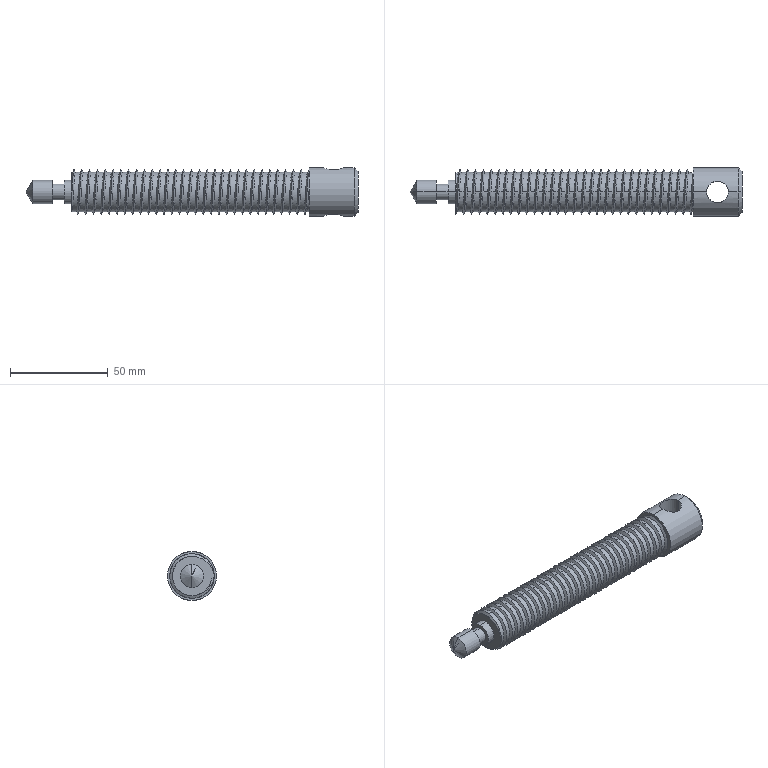Part | SolidWorks | features Chamfer 1, Helix 1, ICE 1, Revolution 1, Sweep 1 | 1 solid | 84 faces | box 169.464 x 25 x 25 mm | volume 51868 mm3 | cylinder 73 | plane 5 | cone 4 | spline 2 | commonest cylinder face diameters 20 x63 12 x4 8 x2 11 x2 25 x2